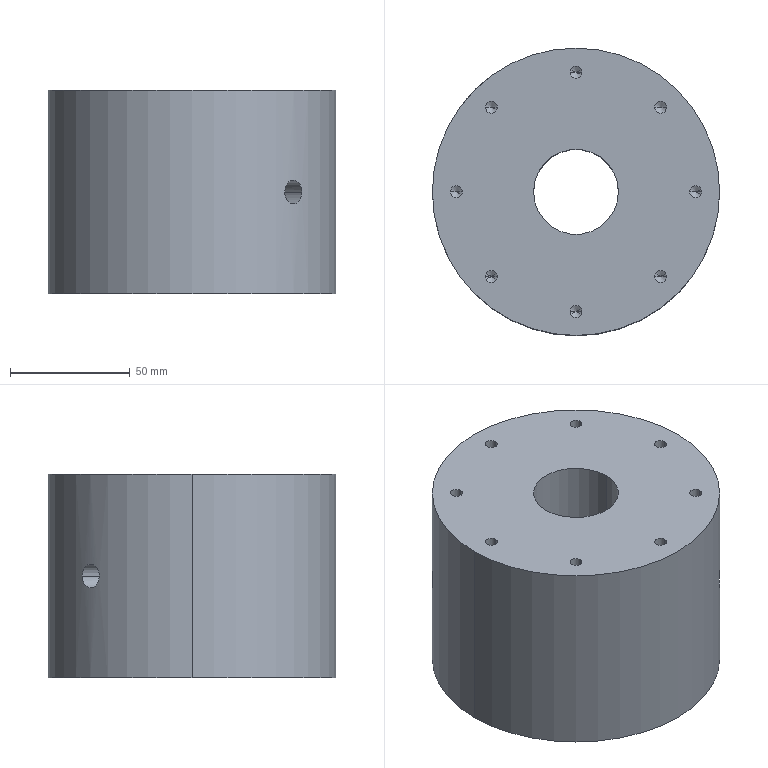Part | SolidWorks | features 3DProfileFeature 2, CirPattern 2, HoleWzd 2, Extrusion 1, ICE 1 | 1 solid | 58 faces | box 120 x 120 x 85 mm | volume 867746 mm3 | cylinder 32 | cone 24 | plane 2 | commonest cylinder face diameters 5 x16 3.3 x8 10 x4 35.5 x2 120 x2